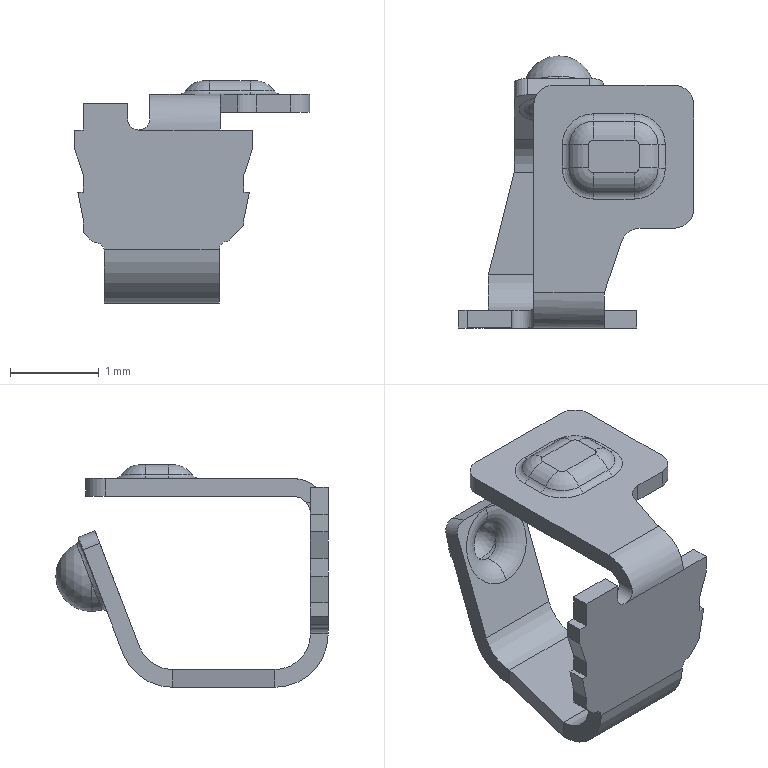Part | NX | 1 solid | 97 faces | box 2.65 x 3.065 x 2.505 mm | volume 2.276 mm3 | plane 40 | cylinder 33 | torus 20 | sphere 4 | commonest cylinder face diameters 0.2 x8 0.12 x4 0.44 x4 0.52 x4 0.6 x4 0.8 x3